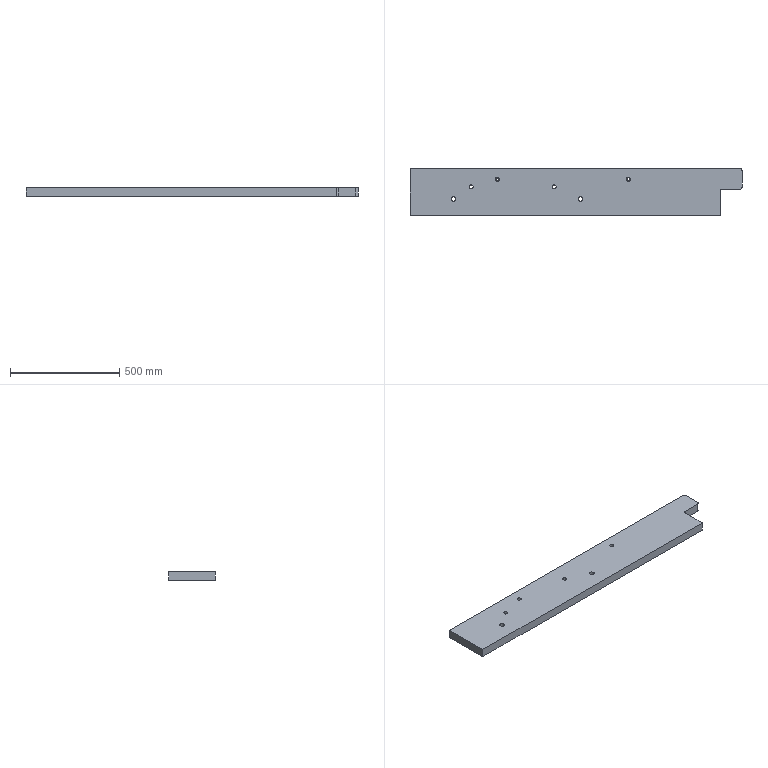Part | SolidWorks | features 3DProfileFeature 2, HoleWzd 2, Extrusion 1, Fillet 1, ICE 1 | 1 solid | 29 faces | box 1520 x 215 x 40 mm | volume 12529786 mm3 | cylinder 19 | plane 10 | commonest cylinder face diameters 18 x8 12 x4 21 x4 20 x3
STEP:
#1=CARTESIAN_POINT('',(1000.,160.,0.));
#2=VERTEX_POINT('',#1);
#3=CARTESIAN_POINT('',(1000.,172.,0.));
#4=VERTEX_POINT('',#3);
#5=CARTESIAN_POINT('',(1000.,166.,0.));
#6=DIRECTION('',(0.,0.,-1.));
#7=DIRECTION('',(0.,1.,0.));
#8=AXIS2_PLACEMENT_3D('',#5,#6,#7);
#9=CIRCLE('',#8,6.);
#10=EDGE_CURVE('',#2,#4,#9,.T.);
#11=ORIENTED_EDGE('',*,*,#10,.T.);
#12=CARTESIAN_POINT('',(1000.,172.,25.));
#13=VERTEX_POINT('',#12);
#14=CARTESIAN_POINT('',(1000.,172.,40.));
#15=DIRECTION('',(0.,0.,1.));
#16=VECTOR('',#15,1000.);
#17=LINE('',#14,#16);
#18=EDGE_CURVE('',#4,#13,#17,.T.);
#19=ORIENTED_EDGE('',*,*,#18,.T.);
#20=CARTESIAN_POINT('',(1000.,160.,25.));
#21=VERTEX_POINT('',#20);
#22=CARTESIAN_POINT('',(1000.,166.,25.));
#23=DIRECTION('',(0.,0.,-1.));
#24=DIRECTION('',(0.,1.,0.));
#25=AXIS2_PLACEMENT_3D('',#22,#23,#24);
#26=CIRCLE('',#25,6.);
#27=EDGE_CURVE('',#21,#13,#26,.T.);
#28=ORIENTED_EDGE('',*,*,#27,.F.);
#29=CARTESIAN_POINT('',(1000.,160.,40.));
#30=DIRECTION('',(0.,0.,1.));
#31=VECTOR('',#30,1000.);
#32=LINE('',#29,#31);
#33=EDGE_CURVE('',#2,#21,#32,.T.);
#34=ORIENTED_EDGE('',*,*,#33,.F.);
#35=EDGE_LOOP('',(#11,#19,#28,#34));
#36=FACE_OUTER_BOUND('',#35,.T.);
#37=CARTESIAN_POINT('',(1000.,166.,40.));
#38=DIRECTION('',(0.,0.,1.));
#39=DIRECTION('',(0.,-1.,0.));
#40=AXIS2_PLACEMENT_3D('',#37,#38,#39);
#41=CYLINDRICAL_SURFACE('',#40,6.);
#42=ADVANCED_FACE('',(#36),#41,.F.);
#43=CARTESIAN_POINT('',(400.,160.,0.));
#44=VERTEX_POINT('',#43);
#45=CARTESIAN_POINT('',(400.,172.,0.));
#46=VERTEX_POINT('',#45);
#47=CARTESIAN_POINT('',(400.,166.,0.));
#48=DIRECTION('',(0.,0.,-1.));
#49=DIRECTION('',(0.,1.,0.));
#50=AXIS2_PLACEMENT_3D('',#47,#48,#49);
#51=CIRCLE('',#50,6.);
#52=EDGE_CURVE('',#44,#46,#51,.T.);
#53=ORIENTED_EDGE('',*,*,#52,.T.);
#54=CARTESIAN_POINT('',(400.,172.,25.));
#55=VERTEX_POINT('',#54);
#56=CARTESIAN_POINT('',(400.,172.,25.));
#57=DIRECTION('',(0.,0.,1.));
#58=VECTOR('',#57,1000.);
#59=LINE('',#56,#58);
#60=EDGE_CURVE('',#46,#55,#59,.T.);
#61=ORIENTED_EDGE('',*,*,#60,.T.);
#62=CARTESIAN_POINT('',(400.,160.,25.));
#63=VERTEX_POINT('',#62);
#64=CARTESIAN_POINT('',(400.,166.,25.));
#65=DIRECTION('',(0.,0.,1.));
#66=DIRECTION('',(0.,-1.,0.));
#67=AXIS2_PLACEMENT_3D('',#64,#65,#66);
#68=CIRCLE('',#67,6.);
#69=EDGE_CURVE('',#55,#63,#68,.T.);
#70=ORIENTED_EDGE('',*,*,#69,.T.);
#71=CARTESIAN_POINT('',(400.,160.,25.));
#72=DIRECTION('',(0.,0.,1.));
#73=VECTOR('',#72,1000.);
#74=LINE('',#71,#73);
#75=EDGE_CURVE('',#44,#63,#74,.T.);
#76=ORIENTED_EDGE('',*,*,#75,.F.);
#77=EDGE_LOOP('',(#53,#61,#70,#76));
#78=FACE_OUTER_BOUND('',#77,.T.);
#79=CARTESIAN_POINT('',(400.,166.,25.));
#80=DIRECTION('',(0.,0.,1.));
#81=DIRECTION('',(0.,-1.,0.));
#82=AXIS2_PLACEMENT_3D('',#79,#80,#81);
#83=CYLINDRICAL_SURFACE('',#82,6.);
#84=ADVANCED_FACE('',(#78),#83,.F.);
#85=CARTESIAN_POINT('',(790.5,75.,0.));
#86=VERTEX_POINT('',#85);
#87=CARTESIAN_POINT('',(769.5,75.,0.));
#88=VERTEX_POINT('',#87);
#89=CARTESIAN_POINT('',(780.,75.,0.));
#90=DIRECTION('',(0.,0.,-1.));
#91=DIRECTION('',(-1.,0.,0.));
#92=AXIS2_PLACEMENT_3D('',#89,#90,#91);
#93=CIRCLE('',#92,10.5);
#94=EDGE_CURVE('',#86,#88,#93,.T.);
#95=ORIENTED_EDGE('',*,*,#94,.T.);
#96=CARTESIAN_POINT('',(769.5,75.,40.));
#97=VERTEX_POINT('',#96);
#98=CARTESIAN_POINT('',(769.5,75.,40.));
#99=DIRECTION('',(0.,0.,1.));
#100=VECTOR('',#99,1000.);
#101=LINE('',#98,#100);
#102=EDGE_CURVE('',#88,#97,#101,.T.);
#103=ORIENTED_EDGE('',*,*,#102,.T.);
#104=CARTESIAN_POINT('',(790.5,75.,40.));
#105=VERTEX_POINT('',#104);
#106=CARTESIAN_POINT('',(780.,75.,40.));
#107=DIRECTION('',(0.,0.,1.));
#108=DIRECTION('',(1.,0.,0.));
#109=AXIS2_PLACEMENT_3D('',#106,#107,#108);
#110=CIRCLE('',#109,10.5);
#111=EDGE_CURVE('',#97,#105,#110,.T.);
#112=ORIENTED_EDGE('',*,*,#111,.T.);
#113=CARTESIAN_POINT('',(790.5,75.,40.));
#114=DIRECTION('',(0.,0.,1.));
#115=VECTOR('',#114,1000.);
#116=LINE('',#113,#115);
#117=EDGE_CURVE('',#86,#105,#116,.T.);
#118=ORIENTED_EDGE('',*,*,#117,.F.);
#119=EDGE_LOOP('',(#95,#103,#112,#118));
#120=FACE_OUTER_BOUND('',#119,.T.);
#121=CARTESIAN_POINT('',(780.,75.,40.));
#122=DIRECTION('',(0.,0.,1.));
#123=DIRECTION('',(1.,0.,0.));
#124=AXIS2_PLACEMENT_3D('',#121,#122,#123);
#125=CYLINDRICAL_SURFACE('',#124,10.5);
#126=ADVANCED_FACE('',(#120),#125,.F.);
#127=CARTESIAN_POINT('',(210.5,75.,0.));
#128=VERTEX_POINT('',#127);
#129=CARTESIAN_POINT('',(189.5,75.,0.));
#130=VERTEX_POINT('',#129);
#131=CARTESIAN_POINT('',(200.,75.,0.));
#132=DIRECTION('',(0.,0.,-1.));
#133=DIRECTION('',(-1.,0.,0.));
#134=AXIS2_PLACEMENT_3D('',#131,#132,#133);
#135=CIRCLE('',#134,10.5);
#136=EDGE_CURVE('',#128,#130,#135,.T.);
#137=ORIENTED_EDGE('',*,*,#136,.T.);
#138=CARTESIAN_POINT('',(189.5,75.,40.));
#139=VERTEX_POINT('',#138);
#140=CARTESIAN_POINT('',(189.5,75.,40.));
#141=DIRECTION('',(0.,0.,1.));
#142=VECTOR('',#141,1000.);
#143=LINE('',#140,#142);
#144=EDGE_CURVE('',#130,#139,#143,.T.);
#145=ORIENTED_EDGE('',*,*,#144,.T.);
#146=CARTESIAN_POINT('',(210.5,75.,40.));
#147=VERTEX_POINT('',#146);
#148=CARTESIAN_POINT('',(200.,75.,40.));
#149=DIRECTION('',(0.,0.,1.));
#150=DIRECTION('',(1.,0.,0.));
#151=AXIS2_PLACEMENT_3D('',#148,#149,#150);
#152=CIRCLE('',#151,10.5);
#153=EDGE_CURVE('',#139,#147,#152,.T.);
#154=ORIENTED_EDGE('',*,*,#153,.T.);
#155=CARTESIAN_POINT('',(210.5,75.,40.));
#156=DIRECTION('',(0.,0.,1.));
#157=VECTOR('',#156,1000.);
#158=LINE('',#155,#157);
#159=EDGE_CURVE('',#128,#147,#158,.T.);
#160=ORIENTED_EDGE('',*,*,#159,.F.);
#161=EDGE_LOOP('',(#137,#145,#154,#160));
#162=FACE_OUTER_BOUND('',#161,.T.);
#163=CARTESIAN_POINT('',(200.,75.,40.));
#164=DIRECTION('',(0.,0.,1.));
#165=DIRECTION('',(1.,0.,0.));
#166=AXIS2_PLACEMENT_3D('',#163,#164,#165);
#167=CYLINDRICAL_SURFACE('',#166,10.5);
#168=ADVANCED_FACE('',(#162),#167,.F.);
#169=CARTESIAN_POINT('',(651.,131.,40.));
#170=VERTEX_POINT('',#169);
#171=CARTESIAN_POINT('',(669.,131.,40.));
#172=VERTEX_POINT('',#171);
#173=CARTESIAN_POINT('',(660.,131.,40.));
#174=DIRECTION('',(0.,0.,1.));
#175=DIRECTION('',(1.,0.,0.));
#176=AXIS2_PLACEMENT_3D('',#173,#174,#175);
#177=CIRCLE('',#176,9.);
#178=EDGE_CURVE('',#170,#172,#177,.T.);
#179=ORIENTED_EDGE('',*,*,#178,.T.);
#180=CARTESIAN_POINT('',(669.,131.,0.));
#181=VERTEX_POINT('',#180);
#182=CARTESIAN_POINT('',(669.,131.,40.));
#183=DIRECTION('',(0.,0.,-1.));
#184=VECTOR('',#183,1000.);
#185=LINE('',#182,#184);
#186=EDGE_CURVE('',#172,#181,#185,.T.);
#187=ORIENTED_EDGE('',*,*,#186,.T.);
#188=CARTESIAN_POINT('',(651.,131.,0.));
#189=VERTEX_POINT('',#188);
#190=CARTESIAN_POINT('',(660.,131.,0.));
#191=DIRECTION('',(0.,0.,1.));
#192=DIRECTION('',(1.,0.,0.));
#193=AXIS2_PLACEMENT_3D('',#190,#191,#192);
#194=CIRCLE('',#193,9.);
#195=EDGE_CURVE('',#189,#181,#194,.T.);
#196=ORIENTED_EDGE('',*,*,#195,.F.);
#197=CARTESIAN_POINT('',(651.,131.,40.));
#198=DIRECTION('',(0.,0.,-1.));
#199=VECTOR('',#198,1000.);
#200=LINE('',#197,#199);
#201=EDGE_CURVE('',#170,#189,#200,.T.);
#202=ORIENTED_EDGE('',*,*,#201,.F.);
#203=EDGE_LOOP('',(#179,#187,#196,#202));
#204=FACE_OUTER_BOUND('',#203,.T.);
#205=CARTESIAN_POINT('',(660.,131.,40.));
#206=DIRECTION('',(0.,0.,-1.));
#207=DIRECTION('',(-1.,0.,0.));
#208=AXIS2_PLACEMENT_3D('',#205,#206,#207);
#209=CYLINDRICAL_SURFACE('',#208,9.);
#210=ADVANCED_FACE('',(#204),#209,.F.);
#211=CARTESIAN_POINT('',(271.,131.,40.));
#212=VERTEX_POINT('',#211);
#213=CARTESIAN_POINT('',(289.,131.,40.));
#214=VERTEX_POINT('',#213);
#215=CARTESIAN_POINT('',(280.,131.,40.));
#216=DIRECTION('',(0.,0.,1.));
#217=DIRECTION('',(1.,0.,0.));
#218=AXIS2_PLACEMENT_3D('',#215,#216,#217);
#219=CIRCLE('',#218,9.);
#220=EDGE_CURVE('',#212,#214,#219,.T.);
#221=ORIENTED_EDGE('',*,*,#220,.T.);
#222=CARTESIAN_POINT('',(289.,131.,0.));
#223=VERTEX_POINT('',#222);
#224=CARTESIAN_POINT('',(289.,131.,40.));
#225=DIRECTION('',(0.,0.,-1.));
#226=VECTOR('',#225,1000.);
#227=LINE('',#224,#226);
#228=EDGE_CURVE('',#214,#223,#227,.T.);
#229=ORIENTED_EDGE('',*,*,#228,.T.);
#230=CARTESIAN_POINT('',(271.,131.,0.));
#231=VERTEX_POINT('',#230);
#232=CARTESIAN_POINT('',(280.,131.,0.));
#233=DIRECTION('',(0.,0.,1.));
#234=DIRECTION('',(1.,0.,0.));
#235=AXIS2_PLACEMENT_3D('',#232,#233,#234);
#236=CIRCLE('',#235,9.);
#237=EDGE_CURVE('',#231,#223,#236,.T.);
#238=ORIENTED_EDGE('',*,*,#237,.F.);
#239=CARTESIAN_POINT('',(271.,131.,40.));
#240=DIRECTION('',(0.,0.,-1.));
#241=VECTOR('',#240,1000.);
#242=LINE('',#239,#241);
#243=EDGE_CURVE('',#212,#231,#242,.T.);
#244=ORIENTED_EDGE('',*,*,#243,.F.);
#245=EDGE_LOOP('',(#221,#229,#238,#244));
#246=FACE_OUTER_BOUND('',#245,.T.);
#247=CARTESIAN_POINT('',(280.,131.,40.));
#248=DIRECTION('',(0.,0.,-1.));
#249=DIRECTION('',(-1.,0.,0.));
#250=AXIS2_PLACEMENT_3D('',#247,#248,#249);
#251=CYLINDRICAL_SURFACE('',#250,9.);
#252=ADVANCED_FACE('',(#246),#251,.F.);
#253=CARTESIAN_POINT('',(991.,166.,40.));
#254=VERTEX_POINT('',#253);
#255=CARTESIAN_POINT('',(1009.,166.,40.));
#256=VERTEX_POINT('',#255);
#257=CARTESIAN_POINT('',(1000.,166.,40.));
#258=DIRECTION('',(0.,0.,1.));
#259=DIRECTION('',(1.,0.,0.));
#260=AXIS2_PLACEMENT_3D('',#257,#258,#259);
#261=CIRCLE('',#260,9.);
#262=EDGE_CURVE('',#254,#256,#261,.T.);
#263=ORIENTED_EDGE('',*,*,#262,.T.);
#264=CARTESIAN_POINT('',(1009.,166.,25.));
#265=VERTEX_POINT('',#264);
#266=CARTESIAN_POINT('',(1009.,166.,40.));
#267=DIRECTION('',(0.,0.,-1.));
#268=VECTOR('',#267,1000.);
#269=LINE('',#266,#268);
#270=EDGE_CURVE('',#256,#265,#269,.T.);
#271=ORIENTED_EDGE('',*,*,#270,.T.);
#272=CARTESIAN_POINT('',(991.,166.,25.));
#273=VERTEX_POINT('',#272);
#274=CARTESIAN_POINT('',(1000.,166.,25.));
#275=DIRECTION('',(0.,0.,-1.));
#276=DIRECTION('',(0.,1.,0.));
#277=AXIS2_PLACEMENT_3D('',#274,#275,#276);
#278=CIRCLE('',#277,9.);
#279=EDGE_CURVE('',#265,#273,#278,.T.);
#280=ORIENTED_EDGE('',*,*,#279,.T.);
#281=CARTESIAN_POINT('',(991.,166.,40.));
#282=DIRECTION('',(0.,0.,-1.));
#283=VECTOR('',#282,1000.);
#284=LINE('',#281,#283);
#285=EDGE_CURVE('',#254,#273,#284,.T.);
#286=ORIENTED_EDGE('',*,*,#285,.F.);
#287=EDGE_LOOP('',(#263,#271,#280,#286));
#288=FACE_OUTER_BOUND('',#287,.T.);
#289=CARTESIAN_POINT('',(1000.,166.,40.));
#290=DIRECTION('',(0.,0.,-1.));
#291=DIRECTION('',(-1.,0.,0.));
#292=AXIS2_PLACEMENT_3D('',#289,#290,#291);
#293=CYLINDRICAL_SURFACE('',#292,9.);
#294=ADVANCED_FACE('',(#288),#293,.F.);
#295=CARTESIAN_POINT('',(391.,166.,40.));
#296=VERTEX_POINT('',#295);
#297=CARTESIAN_POINT('',(409.,166.,40.));
#298=VERTEX_POINT('',#297);
#299=CARTESIAN_POINT('',(400.,166.,40.));
#300=DIRECTION('',(0.,0.,1.));
#301=DIRECTION('',(1.,0.,0.));
#302=AXIS2_PLACEMENT_3D('',#299,#300,#301);
#303=CIRCLE('',#302,9.);
#304=EDGE_CURVE('',#296,#298,#303,.T.);
#305=ORIENTED_EDGE('',*,*,#304,.T.);
#306=CARTESIAN_POINT('',(409.,166.,25.));
#307=VERTEX_POINT('',#306);
#308=CARTESIAN_POINT('',(409.,166.,40.));
#309=DIRECTION('',(0.,0.,-1.));
#310=VECTOR('',#309,1000.);
#311=LINE('',#308,#310);
#312=EDGE_CURVE('',#298,#307,#311,.T.);
#313=ORIENTED_EDGE('',*,*,#312,.T.);
#314=CARTESIAN_POINT('',(391.,166.,25.));
#315=VERTEX_POINT('',#314);
#316=CARTESIAN_POINT('',(400.,166.,25.));
#317=DIRECTION('',(0.,0.,-1.));
#318=DIRECTION('',(0.,1.,0.));
#319=AXIS2_PLACEMENT_3D('',#316,#317,#318);
#320=CIRCLE('',#319,9.);
#321=EDGE_CURVE('',#307,#315,#320,.T.);
#322=ORIENTED_EDGE('',*,*,#321,.T.);
#323=CARTESIAN_POINT('',(391.,166.,40.));
#324=DIRECTION('',(0.,0.,-1.));
#325=VECTOR('',#324,1000.);
#326=LINE('',#323,#325);
#327=EDGE_CURVE('',#296,#315,#326,.T.);
#328=ORIENTED_EDGE('',*,*,#327,.F.);
#329=EDGE_LOOP('',(#305,#313,#322,#328));
#330=FACE_OUTER_BOUND('',#329,.T.);
#331=CARTESIAN_POINT('',(400.,166.,40.));
#332=DIRECTION('',(0.,0.,-1.));
#333=DIRECTION('',(-1.,0.,0.));
#334=AXIS2_PLACEMENT_3D('',#331,#332,#333);
#335=CYLINDRICAL_SURFACE('',#334,9.);
#336=ADVANCED_FACE('',(#330),#335,.F.);
#337=ORIENTED_EDGE('',*,*,#312,.F.);
#338=CARTESIAN_POINT('',(400.,166.,40.));
#339=DIRECTION('',(0.,0.,1.));
#340=DIRECTION('',(1.,0.,0.));
#341=AXIS2_PLACEMENT_3D('',#338,#339,#340);
#342=CIRCLE('',#341,9.);
#343=EDGE_CURVE('',#298,#296,#342,.T.);
#344=ORIENTED_EDGE('',*,*,#343,.T.);
#345=ORIENTED_EDGE('',*,*,#327,.T.);
#346=CARTESIAN_POINT('',(400.,166.,25.));
#347=DIRECTION('',(0.,0.,-1.));
#348=DIRECTION('',(0.,1.,0.));
#349=AXIS2_PLACEMENT_3D('',#346,#347,#348);
#350=CIRCLE('',#349,9.);
#351=EDGE_CURVE('',#315,#307,#350,.T.);
#352=ORIENTED_EDGE('',*,*,#351,.T.);
#353=EDGE_LOOP('',(#337,#344,#345,#352));
#354=FACE_OUTER_BOUND('',#353,.T.);
#355=CARTESIAN_POINT('',(400.,166.,40.));
#356=DIRECTION('',(0.,0.,-1.));
#357=DIRECTION('',(-1.,0.,0.));
#358=AXIS2_PLACEMENT_3D('',#355,#356,#357);
#359=CYLINDRICAL_SURFACE('',#358,9.);
#360=ADVANCED_FACE('',(#354),#359,.F.);
#361=ORIENTED_EDGE('',*,*,#270,.F.);
#362=CARTESIAN_POINT('',(1000.,166.,40.));
#363=DIRECTION('',(0.,0.,1.));
#364=DIRECTION('',(1.,0.,0.));
#365=AXIS2_PLACEMENT_3D('',#362,#363,#364);
#366=CIRCLE('',#365,9.);
#367=EDGE_CURVE('',#256,#254,#366,.T.);
#368=ORIENTED_EDGE('',*,*,#367,.T.);
#369=ORIENTED_EDGE('',*,*,#285,.T.);
#370=CARTESIAN_POINT('',(1000.,166.,25.));
#371=DIRECTION('',(0.,0.,-1.));
#372=DIRECTION('',(0.,1.,0.));
#373=AXIS2_PLACEMENT_3D('',#370,#371,#372);
#374=CIRCLE('',#373,9.);
#375=EDGE_CURVE('',#273,#265,#374,.T.);
#376=ORIENTED_EDGE('',*,*,#375,.T.);
#377=EDGE_LOOP('',(#361,#368,#369,#376));
#378=FACE_OUTER_BOUND('',#377,.T.);
#379=CARTESIAN_POINT('',(1000.,166.,40.));
#380=DIRECTION('',(0.,0.,-1.));
#381=DIRECTION('',(-1.,0.,0.));
#382=AXIS2_PLACEMENT_3D('',#379,#380,#381);
#383=CYLINDRICAL_SURFACE('',#382,9.);
#384=ADVANCED_FACE('',(#378),#383,.F.);
#385=CARTESIAN_POINT('',(780.,75.,40.));
#386=DIRECTION('',(0.,0.,1.));
#387=DIRECTION('',(1.,0.,0.));
#388=AXIS2_PLACEMENT_3D('',#385,#386,#387);
#389=CIRCLE('',#388,10.5);
#390=EDGE_CURVE('',#105,#97,#389,.T.);
#391=ORIENTED_EDGE('',*,*,#390,.F.);
#392=ORIENTED_EDGE('',*,*,#111,.F.);
#393=EDGE_LOOP('',(#391,#392));
#394=FACE_BOUND('',#393,.T.);
#395=CARTESIAN_POINT('',(200.,75.,40.));
#396=DIRECTION('',(0.,0.,1.));
#397=DIRECTION('',(1.,0.,0.));
#398=AXIS2_PLACEMENT_3D('',#395,#396,#397);
#399=CIRCLE('',#398,10.5);
#400=EDGE_CURVE('',#147,#139,#399,.T.);
#401=ORIENTED_EDGE('',*,*,#400,.F.);
#402=ORIENTED_EDGE('',*,*,#153,.F.);
#403=EDGE_LOOP('',(#401,#402));
#404=FACE_BOUND('',#403,.T.);
#405=CARTESIAN_POINT('',(1520.,130.,40.));
#406=VERTEX_POINT('',#405);
#407=CARTESIAN_POINT('',(1520.,205.,40.));
#408=VERTEX_POINT('',#407);
#409=CARTESIAN_POINT('',(1520.,120.,40.));
#410=DIRECTION('',(0.,1.,0.));
#411=VECTOR('',#410,1000.);
#412=LINE('',#409,#411);
#413=EDGE_CURVE('',#406,#408,#412,.T.);
#414=ORIENTED_EDGE('',*,*,#413,.T.);
#415=CARTESIAN_POINT('',(1510.,215.,40.));
#416=VERTEX_POINT('',#415);
#417=CARTESIAN_POINT('',(1510.,205.,40.));
#418=DIRECTION('',(0.,0.,1.));
#419=DIRECTION('',(-1.,0.,0.));
#420=AXIS2_PLACEMENT_3D('',#417,#418,#419);
#421=CIRCLE('',#420,10.);
#422=EDGE_CURVE('',#408,#416,#421,.T.);
#423=ORIENTED_EDGE('',*,*,#422,.T.);
#424=CARTESIAN_POINT('',(0.,215.,40.));
#425=VERTEX_POINT('',#424);
#426=CARTESIAN_POINT('',(0.,215.,40.));
#427=DIRECTION('',(-1.,0.,0.));
#428=VECTOR('',#427,1000.);
#429=LINE('',#426,#428);
#430=EDGE_CURVE('',#416,#425,#429,.T.);
#431=ORIENTED_EDGE('',*,*,#430,.T.);
#432=CARTESIAN_POINT('',(0.,0.,40.));
#433=VERTEX_POINT('',#432);
#434=CARTESIAN_POINT('',(0.,0.,40.));
#435=DIRECTION('',(0.,-1.,0.));
#436=VECTOR('',#435,1000.);
#437=LINE('',#434,#436);
#438=EDGE_CURVE('',#425,#433,#437,.T.);
#439=ORIENTED_EDGE('',*,*,#438,.T.);
#440=CARTESIAN_POINT('',(1420.,0.,40.));
#441=VERTEX_POINT('',#440);
#442=CARTESIAN_POINT('',(0.,0.,40.));
#443=DIRECTION('',(1.,0.,0.));
#444=VECTOR('',#443,1000.);
#445=LINE('',#442,#444);
#446=EDGE_CURVE('',#433,#441,#445,.T.);
#447=ORIENTED_EDGE('',*,*,#446,.T.);
#448=CARTESIAN_POINT('',(1420.,110.,40.));
#449=VERTEX_POINT('',#448);
#450=CARTESIAN_POINT('',(1420.,0.,40.));
#451=DIRECTION('',(0.,1.,0.));
#452=VECTOR('',#451,1000.);
#453=LINE('',#450,#452);
#454=EDGE_CURVE('',#441,#449,#453,.T.);
#455=ORIENTED_EDGE('',*,*,#454,.T.);
#456=CARTESIAN_POINT('',(1430.,120.,40.));
#457=VERTEX_POINT('',#456);
#458=CARTESIAN_POINT('',(1430.,110.,40.));
#459=DIRECTION('',(0.,0.,-1.));
#460=DIRECTION('',(-1.,0.,0.));
#461=AXIS2_PLACEMENT_3D('',#458,#459,#460);
#462=CIRCLE('',#461,10.);
#463=EDGE_CURVE('',#449,#457,#462,.T.);
#464=ORIENTED_EDGE('',*,*,#463,.T.);
#465=CARTESIAN_POINT('',(1510.,120.,40.));
#466=VERTEX_POINT('',#465);
#467=CARTESIAN_POINT('',(1420.,120.,40.));
#468=DIRECTION('',(1.,0.,0.));
#469=VECTOR('',#468,1000.);
#470=LINE('',#467,#469);
#471=EDGE_CURVE('',#457,#466,#470,.T.);
#472=ORIENTED_EDGE('',*,*,#471,.T.);
#473=CARTESIAN_POINT('',(1510.,130.,40.));
#474=DIRECTION('',(0.,0.,1.));
#475=DIRECTION('',(-1.,0.,0.));
#476=AXIS2_PLACEMENT_3D('',#473,#474,#475);
#477=CIRCLE('',#476,10.);
#478=EDGE_CURVE('',#466,#406,#477,.T.);
#479=ORIENTED_EDGE('',*,*,#478,.T.);
#480=EDGE_LOOP('',(#414,#423,#431,#439,#447,#455,#464,#472,#479));
#481=FACE_OUTER_BOUND('',#480,.T.);
#482=ORIENTED_EDGE('',*,*,#304,.F.);
#483=ORIENTED_EDGE('',*,*,#343,.F.);
#484=EDGE_LOOP('',(#482,#483));
#485=FACE_BOUND('',#484,.T.);
#486=ORIENTED_EDGE('',*,*,#220,.F.);
#487=CARTESIAN_POINT('',(280.,131.,40.));
#488=DIRECTION('',(0.,0.,1.));
#489=DIRECTION('',(1.,0.,0.));
#490=AXIS2_PLACEMENT_3D('',#487,#488,#489);
#491=CIRCLE('',#490,9.);
#492=EDGE_CURVE('',#214,#212,#491,.T.);
#493=ORIENTED_EDGE('',*,*,#492,.F.);
#494=EDGE_LOOP('',(#486,#493));
#495=FACE_BOUND('',#494,.T.);
#496=ORIENTED_EDGE('',*,*,#178,.F.);
#497=CARTESIAN_POINT('',(660.,131.,40.));
#498=DIRECTION('',(0.,0.,1.));
#499=DIRECTION('',(1.,0.,0.));
#500=AXIS2_PLACEMENT_3D('',#497,#498,#499);
#501=CIRCLE('',#500,9.);
#502=EDGE_CURVE('',#172,#170,#501,.T.);
#503=ORIENTED_EDGE('',*,*,#502,.F.);
#504=EDGE_LOOP('',(#496,#503));
#505=FACE_BOUND('',#504,.T.);
#506=ORIENTED_EDGE('',*,*,#262,.F.);
#507=ORIENTED_EDGE('',*,*,#367,.F.);
#508=EDGE_LOOP('',(#506,#507));
#509=FACE_BOUND('',#508,.T.);
#510=CARTESIAN_POINT('',(0.,0.,40.));
#511=DIRECTION('',(0.,0.,-1.));
#512=DIRECTION('',(-1.,0.,0.));
#513=AXIS2_PLACEMENT_3D('',#510,#511,#512);
#514=PLANE('',#513);
#515=ADVANCED_FACE('',(#394,#404,#481,#485,#495,#505,#509),#514,.F.);
#516=ORIENTED_EDGE('',*,*,#10,.F.);
#517=CARTESIAN_POINT('',(1000.,166.,0.));
#518=DIRECTION('',(0.,0.,-1.));
#519=DIRECTION('',(0.,1.,0.));
#520=AXIS2_PLACEMENT_3D('',#517,#518,#519);
#521=CIRCLE('',#520,6.);
#522=EDGE_CURVE('',#4,#2,#521,.T.);
#523=ORIENTED_EDGE('',*,*,#522,.F.);
#524=EDGE_LOOP('',(#516,#523));
#525=FACE_BOUND('',#524,.T.);
#526=ORIENTED_EDGE('',*,*,#52,.F.);
#527=CARTESIAN_POINT('',(400.,166.,0.));
#528=DIRECTION('',(0.,0.,-1.));
#529=DIRECTION('',(0.,1.,0.));
#530=AXIS2_PLACEMENT_3D('',#527,#528,#529);
#531=CIRCLE('',#530,6.);
#532=EDGE_CURVE('',#46,#44,#531,.T.);
#533=ORIENTED_EDGE('',*,*,#532,.F.);
#534=EDGE_LOOP('',(#526,#533));
#535=FACE_BOUND('',#534,.T.);
#536=ORIENTED_EDGE('',*,*,#94,.F.);
#537=CARTESIAN_POINT('',(780.,75.,0.));
#538=DIRECTION('',(0.,0.,-1.));
#539=DIRECTION('',(-1.,0.,0.));
#540=AXIS2_PLACEMENT_3D('',#537,#538,#539);
#541=CIRCLE('',#540,10.5);
#542=EDGE_CURVE('',#88,#86,#541,.T.);
#543=ORIENTED_EDGE('',*,*,#542,.F.);
#544=EDGE_LOOP('',(#536,#543));
#545=FACE_BOUND('',#544,.T.);
#546=ORIENTED_EDGE('',*,*,#136,.F.);
#547=CARTESIAN_POINT('',(200.,75.,0.));
#548=DIRECTION('',(0.,0.,-1.));
#549=DIRECTION('',(-1.,0.,0.));
#550=AXIS2_PLACEMENT_3D('',#547,#548,#549);
#551=CIRCLE('',#550,10.5);
#552=EDGE_CURVE('',#130,#128,#551,.T.);
#553=ORIENTED_EDGE('',*,*,#552,.F.);
#554=EDGE_LOOP('',(#546,#553));
#555=FACE_BOUND('',#554,.T.);
#556=ORIENTED_EDGE('',*,*,#195,.T.);
#557=CARTESIAN_POINT('',(660.,131.,0.));
#558=DIRECTION('',(0.,0.,1.));
#559=DIRECTION('',(1.,0.,0.));
#560=AXIS2_PLACEMENT_3D('',#557,#558,#559);
#561=CIRCLE('',#560,9.);
#562=EDGE_CURVE('',#181,#189,#561,.T.);
#563=ORIENTED_EDGE('',*,*,#562,.T.);
#564=EDGE_LOOP('',(#556,#563));
#565=FACE_BOUND('',#564,.T.);
#566=CARTESIAN_POINT('',(1510.,215.,0.));
#567=VERTEX_POINT('',#566);
#568=CARTESIAN_POINT('',(0.,215.,0.));
#569=VERTEX_POINT('',#568);
#570=CARTESIAN_POINT('',(0.,215.,0.));
#571=DIRECTION('',(-1.,0.,0.));
#572=VECTOR('',#571,1000.);
#573=LINE('',#570,#572);
#574=EDGE_CURVE('',#567,#569,#573,.T.);
#575=ORIENTED_EDGE('',*,*,#574,.F.);
#576=CARTESIAN_POINT('',(1520.,205.,0.));
#577=VERTEX_POINT('',#576);
#578=CARTESIAN_POINT('',(1510.,205.,0.));
#579=DIRECTION('',(0.,0.,-1.));
#580=DIRECTION('',(-1.,0.,0.));
#581=AXIS2_PLACEMENT_3D('',#578,#579,#580);
#582=CIRCLE('',#581,10.);
#583=EDGE_CURVE('',#567,#577,#582,.T.);
#584=ORIENTED_EDGE('',*,*,#583,.T.);
#585=CARTESIAN_POINT('',(1520.,130.,0.));
#586=VERTEX_POINT('',#585);
#587=CARTESIAN_POINT('',(1520.,120.,0.));
#588=DIRECTION('',(0.,1.,0.));
#589=VECTOR('',#588,1000.);
#590=LINE('',#587,#589);
#591=EDGE_CURVE('',#586,#577,#590,.T.);
#592=ORIENTED_EDGE('',*,*,#591,.F.);
#593=CARTESIAN_POINT('',(1510.,120.,0.));
#594=VERTEX_POINT('',#593);
#595=CARTESIAN_POINT('',(1510.,130.,0.));
#596=DIRECTION('',(0.,0.,-1.));
#597=DIRECTION('',(-1.,0.,0.));
#598=AXIS2_PLACEMENT_3D('',#595,#596,#597);
#599=CIRCLE('',#598,10.);
#600=EDGE_CURVE('',#586,#594,#599,.T.);
#601=ORIENTED_EDGE('',*,*,#600,.T.);
#602=CARTESIAN_POINT('',(1430.,120.,0.));
#603=VERTEX_POINT('',#602);
#604=CARTESIAN_POINT('',(1420.,120.,0.));
#605=DIRECTION('',(1.,0.,0.));
#606=VECTOR('',#605,1000.);
#607=LINE('',#604,#606);
#608=EDGE_CURVE('',#603,#594,#607,.T.);
#609=ORIENTED_EDGE('',*,*,#608,.F.);
#610=CARTESIAN_POINT('',(1420.,110.,0.));
#611=VERTEX_POINT('',#610);
#612=CARTESIAN_POINT('',(1430.,110.,0.));
#613=DIRECTION('',(0.,0.,1.));
#614=DIRECTION('',(-1.,0.,0.));
#615=AXIS2_PLACEMENT_3D('',#612,#613,#614);
#616=CIRCLE('',#615,10.);
#617=EDGE_CURVE('',#603,#611,#616,.T.);
#618=ORIENTED_EDGE('',*,*,#617,.T.);
#619=CARTESIAN_POINT('',(1420.,0.,0.));
#620=VERTEX_POINT('',#619);
#621=CARTESIAN_POINT('',(1420.,0.,0.));
#622=DIRECTION('',(0.,1.,0.));
#623=VECTOR('',#622,1000.);
#624=LINE('',#621,#623);
#625=EDGE_CURVE('',#620,#611,#624,.T.);
#626=ORIENTED_EDGE('',*,*,#625,.F.);
#627=CARTESIAN_POINT('',(0.,0.,0.));
#628=VERTEX_POINT('',#627);
#629=CARTESIAN_POINT('',(0.,0.,0.));
#630=DIRECTION('',(1.,0.,0.));
#631=VECTOR('',#630,1000.);
#632=LINE('',#629,#631);
#633=EDGE_CURVE('',#628,#620,#632,.T.);
#634=ORIENTED_EDGE('',*,*,#633,.F.);
#635=CARTESIAN_POINT('',(0.,0.,0.));
#636=DIRECTION('',(0.,-1.,0.));
#637=VECTOR('',#636,1000.);
#638=LINE('',#635,#637);
#639=EDGE_CURVE('',#569,#628,#638,.T.);
#640=ORIENTED_EDGE('',*,*,#639,.F.);
#641=EDGE_LOOP('',(#575,#584,#592,#601,#609,#618,#626,#634,#640));
#642=FACE_OUTER_BOUND('',#641,.T.);
#643=ORIENTED_EDGE('',*,*,#237,.T.);
#644=CARTESIAN_POINT('',(280.,131.,0.));
#645=DIRECTION('',(0.,0.,1.));
#646=DIRECTION('',(1.,0.,0.));
#647=AXIS2_PLACEMENT_3D('',#644,#645,#646);
#648=CIRCLE('',#647,9.);
#649=EDGE_CURVE('',#223,#231,#648,.T.);
#650=ORIENTED_EDGE('',*,*,#649,.T.);
#651=EDGE_LOOP('',(#643,#650));
#652=FACE_BOUND('',#651,.T.);
#653=CARTESIAN_POINT('',(0.,0.,0.));
#654=DIRECTION('',(0.,0.,-1.));
#655=DIRECTION('',(-1.,0.,0.));
#656=AXIS2_PLACEMENT_3D('',#653,#654,#655);
#657=PLANE('',#656);
#658=ADVANCED_FACE('',(#525,#535,#545,#555,#565,#642,#652),#657,.T.);
#659=ORIENTED_EDGE('',*,*,#639,.T.);
#660=CARTESIAN_POINT('',(0.,0.,40.));
#661=DIRECTION('',(0.,0.,-1.));
#662=VECTOR('',#661,1000.);
#663=LINE('',#660,#662);
#664=EDGE_CURVE('',#433,#628,#663,.T.);
#665=ORIENTED_EDGE('',*,*,#664,.F.);
#666=ORIENTED_EDGE('',*,*,#438,.F.);
#667=CARTESIAN_POINT('',(0.,215.,40.));
#668=DIRECTION('',(0.,0.,-1.));
#669=VECTOR('',#668,1000.);
#670=LINE('',#667,#669);
#671=EDGE_CURVE('',#425,#569,#670,.T.);
#672=ORIENTED_EDGE('',*,*,#671,.T.);
#673=EDGE_LOOP('',(#659,#665,#666,#672));
#674=FACE_OUTER_BOUND('',#673,.T.);
#675=CARTESIAN_POINT('',(0.,0.,40.));
#676=DIRECTION('',(1.,0.,0.));
#677=DIRECTION('',(0.,0.,-1.));
#678=AXIS2_PLACEMENT_3D('',#675,#676,#677);
#679=PLANE('',#678);
#680=ADVANCED_FACE('',(#674),#679,.F.);
#681=ORIENTED_EDGE('',*,*,#633,.T.);
#682=CARTESIAN_POINT('',(1420.,0.,40.));
#683=DIRECTION('',(0.,0.,-1.));
#684=VECTOR('',#683,1000.);
#685=LINE('',#682,#684);
#686=EDGE_CURVE('',#441,#620,#685,.T.);
#687=ORIENTED_EDGE('',*,*,#686,.F.);
#688=ORIENTED_EDGE('',*,*,#446,.F.);
#689=ORIENTED_EDGE('',*,*,#664,.T.);
#690=EDGE_LOOP('',(#681,#687,#688,#689));
#691=FACE_OUTER_BOUND('',#690,.T.);
#692=CARTESIAN_POINT('',(0.,0.,40.));
#693=DIRECTION('',(0.,1.,0.));
#694=DIRECTION('',(0.,0.,1.));
#695=AXIS2_PLACEMENT_3D('',#692,#693,#694);
#696=PLANE('',#695);
#697=ADVANCED_FACE('',(#691),#696,.F.);
#698=ORIENTED_EDGE('',*,*,#625,.T.);
#699=CARTESIAN_POINT('',(1420.,110.,40.));
#700=DIRECTION('',(0.,0.,1.));
#701=VECTOR('',#700,1000.);
#702=LINE('',#699,#701);
#703=EDGE_CURVE('',#611,#449,#702,.T.);
#704=ORIENTED_EDGE('',*,*,#703,.T.);
#705=ORIENTED_EDGE('',*,*,#454,.F.);
#706=ORIENTED_EDGE('',*,*,#686,.T.);
#707=EDGE_LOOP('',(#698,#704,#705,#706));
#708=FACE_OUTER_BOUND('',#707,.T.);
#709=CARTESIAN_POINT('',(1420.,0.,40.));
#710=DIRECTION('',(-1.,0.,0.));
#711=DIRECTION('',(0.,0.,1.));
#712=AXIS2_PLACEMENT_3D('',#709,#710,#711);
#713=PLANE('',#712);
#714=ADVANCED_FACE('',(#708),#713,.F.);
#715=ORIENTED_EDGE('',*,*,#608,.T.);
#716=CARTESIAN_POINT('',(1510.,120.,40.));
#717=DIRECTION('',(0.,0.,1.));
#718=VECTOR('',#717,1000.);
#719=LINE('',#716,#718);
#720=EDGE_CURVE('',#594,#466,#719,.T.);
#721=ORIENTED_EDGE('',*,*,#720,.T.);
#722=ORIENTED_EDGE('',*,*,#471,.F.);
#723=CARTESIAN_POINT('',(1430.,120.,0.));
#724=DIRECTION('',(0.,0.,-1.));
#725=VECTOR('',#724,1000.);
#726=LINE('',#723,#725);
#727=EDGE_CURVE('',#457,#603,#726,.T.);
#728=ORIENTED_EDGE('',*,*,#727,.T.);
#729=EDGE_LOOP('',(#715,#721,#722,#728));
#730=FACE_OUTER_BOUND('',#729,.T.);
#731=CARTESIAN_POINT('',(1420.,120.,40.));
#732=DIRECTION('',(0.,1.,0.));
#733=DIRECTION('',(0.,0.,1.));
#734=AXIS2_PLACEMENT_3D('',#731,#732,#733);
#735=PLANE('',#734);
#736=ADVANCED_FACE('',(#730),#735,.F.);
#737=ORIENTED_EDGE('',*,*,#591,.T.);
#738=CARTESIAN_POINT('',(1520.,205.,40.));
#739=DIRECTION('',(0.,0.,1.));
#740=VECTOR('',#739,1000.);
#741=LINE('',#738,#740);
#742=EDGE_CURVE('',#577,#408,#741,.T.);
#743=ORIENTED_EDGE('',*,*,#742,.T.);
#744=ORIENTED_EDGE('',*,*,#413,.F.);
#745=CARTESIAN_POINT('',(1520.,130.,40.));
#746=DIRECTION('',(0.,0.,-1.));
#747=VECTOR('',#746,1000.);
#748=LINE('',#745,#747);
#749=EDGE_CURVE('',#406,#586,#748,.T.);
#750=ORIENTED_EDGE('',*,*,#749,.T.);
#751=EDGE_LOOP('',(#737,#743,#744,#750));
#752=FACE_OUTER_BOUND('',#751,.T.);
#753=CARTESIAN_POINT('',(1520.,120.,40.));
#754=DIRECTION('',(-1.,0.,0.));
#755=DIRECTION('',(0.,0.,1.));
#756=AXIS2_PLACEMENT_3D('',#753,#754,#755);
#757=PLANE('',#756);
#758=ADVANCED_FACE('',(#752),#757,.F.);
#759=ORIENTED_EDGE('',*,*,#430,.F.);
#760=CARTESIAN_POINT('',(1510.,215.,40.));
#761=DIRECTION('',(0.,0.,-1.));
#762=VECTOR('',#761,1000.);
#763=LINE('',#760,#762);
#764=EDGE_CURVE('',#416,#567,#763,.T.);
#765=ORIENTED_EDGE('',*,*,#764,.T.);
#766=ORIENTED_EDGE('',*,*,#574,.T.);
#767=ORIENTED_EDGE('',*,*,#671,.F.);
#768=EDGE_LOOP('',(#759,#765,#766,#767));
#769=FACE_OUTER_BOUND('',#768,.T.);
#770=CARTESIAN_POINT('',(0.,215.,40.));
#771=DIRECTION('',(0.,-1.,0.));
#772=DIRECTION('',(0.,0.,-1.));
#773=AXIS2_PLACEMENT_3D('',#770,#771,#772);
#774=PLANE('',#773);
#775=ADVANCED_FACE('',(#769),#774,.F.);
#776=ORIENTED_EDGE('',*,*,#228,.F.);
#777=ORIENTED_EDGE('',*,*,#492,.T.);
#778=ORIENTED_EDGE('',*,*,#243,.T.);
#779=ORIENTED_EDGE('',*,*,#649,.F.);
#780=EDGE_LOOP('',(#776,#777,#778,#779));
#781=FACE_OUTER_BOUND('',#780,.T.);
#782=CARTESIAN_POINT('',(280.,131.,40.));
#783=DIRECTION('',(0.,0.,-1.));
#784=DIRECTION('',(-1.,0.,0.));
#785=AXIS2_PLACEMENT_3D('',#782,#783,#784);
#786=CYLINDRICAL_SURFACE('',#785,9.);
#787=ADVANCED_FACE('',(#781),#786,.F.);
#788=ORIENTED_EDGE('',*,*,#186,.F.);
#789=ORIENTED_EDGE('',*,*,#502,.T.);
#790=ORIENTED_EDGE('',*,*,#201,.T.);
#791=ORIENTED_EDGE('',*,*,#562,.F.);
#792=EDGE_LOOP('',(#788,#789,#790,#791));
#793=FACE_OUTER_BOUND('',#792,.T.);
#794=CARTESIAN_POINT('',(660.,131.,40.));
#795=DIRECTION('',(0.,0.,-1.));
#796=DIRECTION('',(-1.,0.,0.));
#797=AXIS2_PLACEMENT_3D('',#794,#795,#796);
#798=CYLINDRICAL_SURFACE('',#797,9.);
#799=ADVANCED_FACE('',(#793),#798,.F.);
#800=ORIENTED_EDGE('',*,*,#144,.F.);
#801=ORIENTED_EDGE('',*,*,#552,.T.);
#802=ORIENTED_EDGE('',*,*,#159,.T.);
#803=ORIENTED_EDGE('',*,*,#400,.T.);
#804=EDGE_LOOP('',(#800,#801,#802,#803));
#805=FACE_OUTER_BOUND('',#804,.T.);
#806=CARTESIAN_POINT('',(200.,75.,40.));
#807=DIRECTION('',(0.,0.,1.));
#808=DIRECTION('',(1.,0.,0.));
#809=AXIS2_PLACEMENT_3D('',#806,#807,#808);
#810=CYLINDRICAL_SURFACE('',#809,10.5);
#811=ADVANCED_FACE('',(#805),#810,.F.);
#812=ORIENTED_EDGE('',*,*,#102,.F.);
#813=ORIENTED_EDGE('',*,*,#542,.T.);
#814=ORIENTED_EDGE('',*,*,#117,.T.);
#815=ORIENTED_EDGE('',*,*,#390,.T.);
#816=EDGE_LOOP('',(#812,#813,#814,#815));
#817=FACE_OUTER_BOUND('',#816,.T.);
#818=CARTESIAN_POINT('',(780.,75.,40.));
#819=DIRECTION('',(0.,0.,1.));
#820=DIRECTION('',(1.,0.,0.));
#821=AXIS2_PLACEMENT_3D('',#818,#819,#820);
#822=CYLINDRICAL_SURFACE('',#821,10.5);
#823=ADVANCED_FACE('',(#817),#822,.F.);
#824=ORIENTED_EDGE('',*,*,#422,.F.);
#825=ORIENTED_EDGE('',*,*,#742,.F.);
#826=ORIENTED_EDGE('',*,*,#583,.F.);
#827=ORIENTED_EDGE('',*,*,#764,.F.);
#828=EDGE_LOOP('',(#824,#825,#826,#827));
#829=FACE_OUTER_BOUND('',#828,.T.);
#830=CARTESIAN_POINT('',(1510.,205.,40.));
#831=DIRECTION('',(0.,0.,-1.));
#832=DIRECTION('',(-1.,0.,0.));
#833=AXIS2_PLACEMENT_3D('',#830,#831,#832);
#834=CYLINDRICAL_SURFACE('',#833,10.);
#835=ADVANCED_FACE('',(#829),#834,.T.);
#836=ORIENTED_EDGE('',*,*,#478,.F.);
#837=ORIENTED_EDGE('',*,*,#720,.F.);
#838=ORIENTED_EDGE('',*,*,#600,.F.);
#839=ORIENTED_EDGE('',*,*,#749,.F.);
#840=EDGE_LOOP('',(#836,#837,#838,#839));
#841=FACE_OUTER_BOUND('',#840,.T.);
#842=CARTESIAN_POINT('',(1510.,130.,40.));
#843=DIRECTION('',(0.,0.,-1.));
#844=DIRECTION('',(-1.,0.,0.));
#845=AXIS2_PLACEMENT_3D('',#842,#843,#844);
#846=CYLINDRICAL_SURFACE('',#845,10.);
#847=ADVANCED_FACE('',(#841),#846,.T.);
#848=ORIENTED_EDGE('',*,*,#463,.F.);
#849=ORIENTED_EDGE('',*,*,#703,.F.);
#850=ORIENTED_EDGE('',*,*,#617,.F.);
#851=ORIENTED_EDGE('',*,*,#727,.F.);
#852=EDGE_LOOP('',(#848,#849,#850,#851));
#853=FACE_OUTER_BOUND('',#852,.T.);
#854=CARTESIAN_POINT('',(1430.,110.,40.));
#855=DIRECTION('',(0.,0.,1.));
#856=DIRECTION('',(1.,0.,0.));
#857=AXIS2_PLACEMENT_3D('',#854,#855,#856);
#858=CYLINDRICAL_SURFACE('',#857,10.);
#859=ADVANCED_FACE('',(#853),#858,.F.);
#860=ORIENTED_EDGE('',*,*,#27,.T.);
#861=CARTESIAN_POINT('',(1000.,166.,25.));
#862=DIRECTION('',(0.,0.,-1.));
#863=DIRECTION('',(0.,1.,0.));
#864=AXIS2_PLACEMENT_3D('',#861,#862,#863);
#865=CIRCLE('',#864,6.);
#866=EDGE_CURVE('',#13,#21,#865,.T.);
#867=ORIENTED_EDGE('',*,*,#866,.T.);
#868=EDGE_LOOP('',(#860,#867));
#869=FACE_BOUND('',#868,.T.);
#870=ORIENTED_EDGE('',*,*,#375,.F.);
#871=ORIENTED_EDGE('',*,*,#279,.F.);
#872=EDGE_LOOP('',(#870,#871));
#873=FACE_OUTER_BOUND('',#872,.T.);
#874=CARTESIAN_POINT('',(1000.,166.,25.));
#875=DIRECTION('',(0.,0.,-1.));
#876=DIRECTION('',(0.,1.,0.));
#877=AXIS2_PLACEMENT_3D('',#874,#875,#876);
#878=PLANE('',#877);
#879=ADVANCED_FACE('',(#869,#873),#878,.F.);
#880=CARTESIAN_POINT('',(400.,166.,25.));
#881=DIRECTION('',(0.,0.,1.));
#882=DIRECTION('',(0.,-1.,0.));
#883=AXIS2_PLACEMENT_3D('',#880,#881,#882);
#884=CIRCLE('',#883,6.);
#885=EDGE_CURVE('',#63,#55,#884,.T.);
#886=ORIENTED_EDGE('',*,*,#885,.F.);
#887=ORIENTED_EDGE('',*,*,#69,.F.);
#888=EDGE_LOOP('',(#886,#887));
#889=FACE_BOUND('',#888,.T.);
#890=ORIENTED_EDGE('',*,*,#351,.F.);
#891=ORIENTED_EDGE('',*,*,#321,.F.);
#892=EDGE_LOOP('',(#890,#891));
#893=FACE_OUTER_BOUND('',#892,.T.);
#894=CARTESIAN_POINT('',(400.,166.,25.));
#895=DIRECTION('',(0.,0.,-1.));
#896=DIRECTION('',(0.,1.,0.));
#897=AXIS2_PLACEMENT_3D('',#894,#895,#896);
#898=PLANE('',#897);
#899=ADVANCED_FACE('',(#889,#893),#898,.F.);
#900=ORIENTED_EDGE('',*,*,#60,.F.);
#901=ORIENTED_EDGE('',*,*,#532,.T.);
#902=ORIENTED_EDGE('',*,*,#75,.T.);
#903=ORIENTED_EDGE('',*,*,#885,.T.);
#904=EDGE_LOOP('',(#900,#901,#902,#903));
#905=FACE_OUTER_BOUND('',#904,.T.);
#906=CARTESIAN_POINT('',(400.,166.,25.));
#907=DIRECTION('',(0.,0.,1.));
#908=DIRECTION('',(0.,-1.,0.));
#909=AXIS2_PLACEMENT_3D('',#906,#907,#908);
#910=CYLINDRICAL_SURFACE('',#909,6.);
#911=ADVANCED_FACE('',(#905),#910,.F.);
#912=ORIENTED_EDGE('',*,*,#18,.F.);
#913=ORIENTED_EDGE('',*,*,#522,.T.);
#914=ORIENTED_EDGE('',*,*,#33,.T.);
#915=ORIENTED_EDGE('',*,*,#866,.F.);
#916=EDGE_LOOP('',(#912,#913,#914,#915));
#917=FACE_OUTER_BOUND('',#916,.T.);
#918=CARTESIAN_POINT('',(1000.,166.,40.));
#919=DIRECTION('',(0.,0.,1.));
#920=DIRECTION('',(0.,-1.,0.));
#921=AXIS2_PLACEMENT_3D('',#918,#919,#920);
#922=CYLINDRICAL_SURFACE('',#921,6.);
#923=ADVANCED_FACE('',(#917),#922,.F.);
#924=CLOSED_SHELL('',(#42,#84,#126,#168,#210,#252,#294,#336,#360,#384,#515,#658,#680,#697,#714,#736,#758,#775,#787,#799,#811,#823,#835,#847,#859,#879,#899,#911,#923));
#925=MANIFOLD_SOLID_BREP('',#924);
#926=CARTESIAN_POINT('',(0.,0.,0.));
#927=DIRECTION('',(0.,0.,1.));
#928=DIRECTION('',(1.,0.,0.));
#929=AXIS2_PLACEMENT_3D('',#926,#927,#928);
#930=(LENGTH_UNIT()NAMED_UNIT(*)SI_UNIT(.MILLI.,.METRE.));
#931=UNCERTAINTY_MEASURE_WITH_UNIT(LENGTH_MEASURE(0.00001),#930,'','');
#932=(NAMED_UNIT(*)PLANE_ANGLE_UNIT()SI_UNIT($,.RADIAN.));
#933=(NAMED_UNIT(*)SI_UNIT($,.STERADIAN.)SOLID_ANGLE_UNIT());
#934=(GEOMETRIC_REPRESENTATION_CONTEXT(3)GLOBAL_UNCERTAINTY_ASSIGNED_CONTEXT((#931))GLOBAL_UNIT_ASSIGNED_CONTEXT((#930,#932,#933))REPRESENTATION_CONTEXT('',''));
#935=ADVANCED_BREP_SHAPE_REPRESENTATION('',(#925,#929),#934);